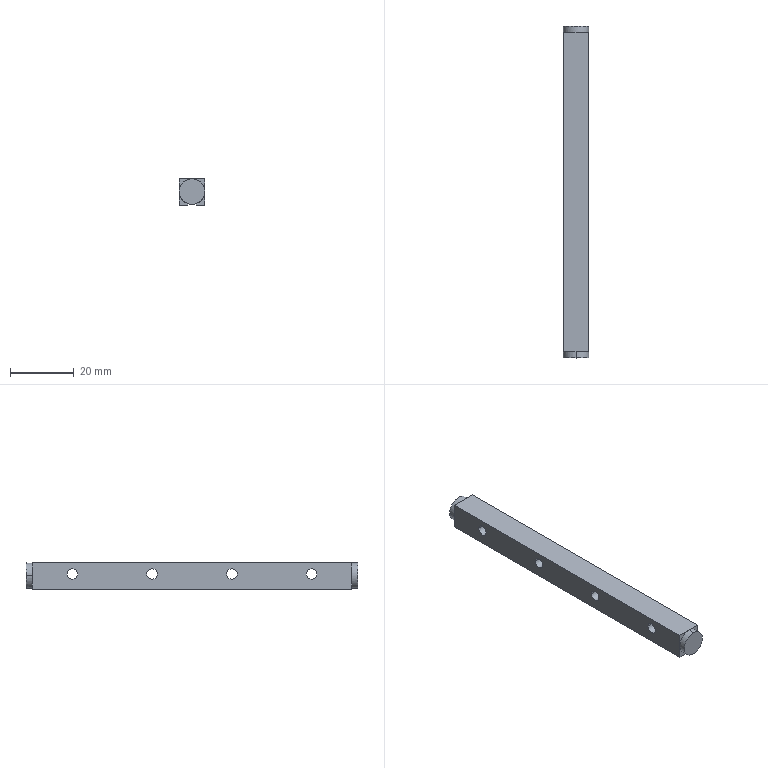Part | NX | 1 solid | 43 faces | box 8 x 104 x 8.3 mm | volume 6121 mm3 | plane 23 | cylinder 20 | commonest cylinder face diameters 3.3 x8 6 x8 8 x4
STEP:
#1=CARTESIAN_POINT('',(4.995,0.,-7.874));
#2=VERTEX_POINT('',#1);
#3=CARTESIAN_POINT('',(8.,0.,-4.));
#4=VERTEX_POINT('',#3);
#5=CARTESIAN_POINT('',(4.,0.,-4.));
#6=DIRECTION('',(0.,-1.,0.));
#7=DIRECTION('',(0.2489,0.,-0.9685));
#8=AXIS2_PLACEMENT_3D('',#5,#6,#7);
#9=CIRCLE('',#8,4.);
#10=EDGE_CURVE('',#2,#4,#9,.T.);
#11=ORIENTED_EDGE('',*,*,#10,.F.);
#12=CARTESIAN_POINT('',(5.421,0.,-8.3));
#13=VERTEX_POINT('',#12);
#14=CARTESIAN_POINT('',(5.421,0.,-8.3));
#15=DIRECTION('',(-0.7071,0.,0.7071));
#16=VECTOR('',#15,1000.);
#17=LINE('',#14,#16);
#18=EDGE_CURVE('',#13,#2,#17,.T.);
#19=ORIENTED_EDGE('',*,*,#18,.F.);
#20=CARTESIAN_POINT('',(8.,0.,-8.3));
#21=VERTEX_POINT('',#20);
#22=CARTESIAN_POINT('',(5.421,0.,-8.3));
#23=DIRECTION('',(1.,0.,0.));
#24=VECTOR('',#23,1000.);
#25=LINE('',#22,#24);
#26=EDGE_CURVE('',#13,#21,#25,.T.);
#27=ORIENTED_EDGE('',*,*,#26,.T.);
#28=CARTESIAN_POINT('',(8.,0.,-8.3));
#29=DIRECTION('',(0.,0.,1.));
#30=VECTOR('',#29,1000.);
#31=LINE('',#28,#30);
#32=EDGE_CURVE('',#21,#4,#31,.T.);
#33=ORIENTED_EDGE('',*,*,#32,.T.);
#34=EDGE_LOOP('',(#11,#19,#27,#33));
#35=FACE_BOUND('',#34,.T.);
#36=CARTESIAN_POINT('',(0.,0.,0.));
#37=DIRECTION('',(0.,1.,0.));
#38=DIRECTION('',(1.,0.,0.));
#39=AXIS2_PLACEMENT_3D('',#36,#37,#38);
#40=PLANE('',#39);
#41=ADVANCED_FACE('',(#35),#40,.F.);
#42=CARTESIAN_POINT('',(4.,-2.,0.));
#43=VERTEX_POINT('',#42);
#44=CARTESIAN_POINT('',(4.,-2.,-8.));
#45=VERTEX_POINT('',#44);
#46=CARTESIAN_POINT('',(4.,-2.,-4.));
#47=DIRECTION('',(0.,1.,0.));
#48=DIRECTION('',(0.,0.,1.));
#49=AXIS2_PLACEMENT_3D('',#46,#47,#48);
#50=CIRCLE('',#49,4.);
#51=EDGE_CURVE('',#43,#45,#50,.T.);
#52=ORIENTED_EDGE('',*,*,#51,.T.);
#53=CARTESIAN_POINT('',(4.,0.,-8.));
#54=VERTEX_POINT('',#53);
#55=CARTESIAN_POINT('',(4.,0.,-8.));
#56=DIRECTION('',(0.,-1.,0.));
#57=VECTOR('',#56,1000.);
#58=LINE('',#55,#57);
#59=EDGE_CURVE('',#45,#54,#58,.F.);
#60=ORIENTED_EDGE('',*,*,#59,.T.);
#61=CARTESIAN_POINT('',(4.,0.,-4.));
#62=DIRECTION('',(0.,-1.,0.));
#63=DIRECTION('',(-0.2489,0.,-0.9685));
#64=AXIS2_PLACEMENT_3D('',#61,#62,#63);
#65=CIRCLE('',#64,4.);
#66=EDGE_CURVE('',#54,#2,#65,.T.);
#67=ORIENTED_EDGE('',*,*,#66,.T.);
#68=ORIENTED_EDGE('',*,*,#10,.T.);
#69=CARTESIAN_POINT('',(4.,0.,0.));
#70=VERTEX_POINT('',#69);
#71=CARTESIAN_POINT('',(4.,0.,-4.));
#72=DIRECTION('',(0.,-1.,0.));
#73=DIRECTION('',(1.,0.,0.));
#74=AXIS2_PLACEMENT_3D('',#71,#72,#73);
#75=CIRCLE('',#74,4.);
#76=EDGE_CURVE('',#4,#70,#75,.T.);
#77=ORIENTED_EDGE('',*,*,#76,.T.);
#78=CARTESIAN_POINT('',(4.,0.,0.));
#79=DIRECTION('',(0.,-1.,0.));
#80=VECTOR('',#79,1000.);
#81=LINE('',#78,#80);
#82=EDGE_CURVE('',#43,#70,#81,.F.);
#83=ORIENTED_EDGE('',*,*,#82,.F.);
#84=EDGE_LOOP('',(#52,#60,#67,#68,#77,#83));
#85=FACE_BOUND('',#84,.T.);
#86=CARTESIAN_POINT('',(4.,0.,-4.));
#87=DIRECTION('',(0.,-1.,0.));
#88=DIRECTION('',(0.,0.,-1.));
#89=AXIS2_PLACEMENT_3D('',#86,#87,#88);
#90=CYLINDRICAL_SURFACE('',#89,4.);
#91=ADVANCED_FACE('',(#85),#90,.T.);
#92=CARTESIAN_POINT('',(4.,0.,-6.879));
#93=VERTEX_POINT('',#92);
#94=CARTESIAN_POINT('',(3.005,0.,-7.874));
#95=VERTEX_POINT('',#94);
#96=CARTESIAN_POINT('',(4.,0.,-6.879));
#97=DIRECTION('',(-0.7071,0.,-0.7071));
#98=VECTOR('',#97,1000.);
#99=LINE('',#96,#98);
#100=EDGE_CURVE('',#93,#95,#99,.T.);
#101=ORIENTED_EDGE('',*,*,#100,.F.);
#102=CARTESIAN_POINT('',(4.995,0.,-7.874));
#103=DIRECTION('',(-0.7071,0.,0.7071));
#104=VECTOR('',#103,1000.);
#105=LINE('',#102,#104);
#106=EDGE_CURVE('',#2,#93,#105,.T.);
#107=ORIENTED_EDGE('',*,*,#106,.F.);
#108=ORIENTED_EDGE('',*,*,#66,.F.);
#109=CARTESIAN_POINT('',(4.,0.,-4.));
#110=DIRECTION('',(0.,-1.,0.));
#111=DIRECTION('',(-0.2489,0.,-0.9685));
#112=AXIS2_PLACEMENT_3D('',#109,#110,#111);
#113=CIRCLE('',#112,4.);
#114=EDGE_CURVE('',#95,#54,#113,.T.);
#115=ORIENTED_EDGE('',*,*,#114,.F.);
#116=EDGE_LOOP('',(#101,#107,#108,#115));
#117=FACE_BOUND('',#116,.T.);
#118=CARTESIAN_POINT('',(0.,0.,0.));
#119=DIRECTION('',(0.,-1.,0.));
#120=DIRECTION('',(0.,0.,-1.));
#121=AXIS2_PLACEMENT_3D('',#118,#119,#120);
#122=PLANE('',#121);
#123=ADVANCED_FACE('',(#117),#122,.F.);
#124=ORIENTED_EDGE('',*,*,#100,.T.);
#125=CARTESIAN_POINT('',(2.579,0.,-8.3));
#126=VERTEX_POINT('',#125);
#127=CARTESIAN_POINT('',(3.005,0.,-7.874));
#128=DIRECTION('',(-0.7071,0.,-0.7071));
#129=VECTOR('',#128,1000.);
#130=LINE('',#127,#129);
#131=EDGE_CURVE('',#95,#126,#130,.T.);
#132=ORIENTED_EDGE('',*,*,#131,.T.);
#133=CARTESIAN_POINT('',(2.579,100.,-8.3));
#134=VERTEX_POINT('',#133);
#135=CARTESIAN_POINT('',(2.579,100.,-8.3));
#136=DIRECTION('',(0.,-1.,0.));
#137=VECTOR('',#136,1000.);
#138=LINE('',#135,#137);
#139=EDGE_CURVE('',#134,#126,#138,.T.);
#140=ORIENTED_EDGE('',*,*,#139,.F.);
#141=CARTESIAN_POINT('',(3.005,100.,-7.874));
#142=VERTEX_POINT('',#141);
#143=CARTESIAN_POINT('',(2.579,100.,-8.3));
#144=DIRECTION('',(0.7071,0.,0.7071));
#145=VECTOR('',#144,1000.);
#146=LINE('',#143,#145);
#147=EDGE_CURVE('',#134,#142,#146,.T.);
#148=ORIENTED_EDGE('',*,*,#147,.T.);
#149=CARTESIAN_POINT('',(4.,100.,-6.879));
#150=VERTEX_POINT('',#149);
#151=CARTESIAN_POINT('',(3.005,100.,-7.874));
#152=DIRECTION('',(0.7071,0.,0.7071));
#153=VECTOR('',#152,1000.);
#154=LINE('',#151,#153);
#155=EDGE_CURVE('',#142,#150,#154,.T.);
#156=ORIENTED_EDGE('',*,*,#155,.T.);
#157=CARTESIAN_POINT('',(4.,0.,-6.879));
#158=DIRECTION('',(0.,1.,0.));
#159=VECTOR('',#158,1000.);
#160=LINE('',#157,#159);
#161=EDGE_CURVE('',#93,#150,#160,.T.);
#162=ORIENTED_EDGE('',*,*,#161,.F.);
#163=EDGE_LOOP('',(#124,#132,#140,#148,#156,#162));
#164=FACE_BOUND('',#163,.T.);
#165=CARTESIAN_POINT('',(1.879,100.,-9.));
#166=DIRECTION('',(-0.7071,0.,0.7071));
#167=DIRECTION('',(0.,1.,0.));
#168=AXIS2_PLACEMENT_3D('',#165,#166,#167);
#169=PLANE('',#168);
#170=ADVANCED_FACE('',(#164),#169,.F.);
#171=ORIENTED_EDGE('',*,*,#106,.T.);
#172=ORIENTED_EDGE('',*,*,#161,.T.);
#173=CARTESIAN_POINT('',(4.995,100.,-7.874));
#174=VERTEX_POINT('',#173);
#175=CARTESIAN_POINT('',(4.,100.,-6.879));
#176=DIRECTION('',(0.7071,0.,-0.7071));
#177=VECTOR('',#176,1000.);
#178=LINE('',#175,#177);
#179=EDGE_CURVE('',#150,#174,#178,.T.);
#180=ORIENTED_EDGE('',*,*,#179,.T.);
#181=CARTESIAN_POINT('',(5.421,100.,-8.3));
#182=VERTEX_POINT('',#181);
#183=CARTESIAN_POINT('',(4.995,100.,-7.874));
#184=DIRECTION('',(0.7071,0.,-0.7071));
#185=VECTOR('',#184,1000.);
#186=LINE('',#183,#185);
#187=EDGE_CURVE('',#174,#182,#186,.T.);
#188=ORIENTED_EDGE('',*,*,#187,.T.);
#189=CARTESIAN_POINT('',(5.421,100.,-8.3));
#190=DIRECTION('',(0.,-1.,0.));
#191=VECTOR('',#190,1000.);
#192=LINE('',#189,#191);
#193=EDGE_CURVE('',#182,#13,#192,.T.);
#194=ORIENTED_EDGE('',*,*,#193,.T.);
#195=ORIENTED_EDGE('',*,*,#18,.T.);
#196=EDGE_LOOP('',(#171,#172,#180,#188,#194,#195));
#197=FACE_BOUND('',#196,.T.);
#198=CARTESIAN_POINT('',(4.,100.,-6.879));
#199=DIRECTION('',(0.7071,0.,0.7071));
#200=DIRECTION('',(0.,-1.,0.));
#201=AXIS2_PLACEMENT_3D('',#198,#199,#200);
#202=PLANE('',#201);
#203=ADVANCED_FACE('',(#197),#202,.F.);
#204=ORIENTED_EDGE('',*,*,#193,.F.);
#205=CARTESIAN_POINT('',(8.,100.,-8.3));
#206=VERTEX_POINT('',#205);
#207=CARTESIAN_POINT('',(5.421,100.,-8.3));
#208=DIRECTION('',(1.,0.,0.));
#209=VECTOR('',#208,1000.);
#210=LINE('',#207,#209);
#211=EDGE_CURVE('',#182,#206,#210,.T.);
#212=ORIENTED_EDGE('',*,*,#211,.T.);
#213=CARTESIAN_POINT('',(8.,100.,-8.3));
#214=DIRECTION('',(0.,-1.,0.));
#215=VECTOR('',#214,1000.);
#216=LINE('',#213,#215);
#217=EDGE_CURVE('',#206,#21,#216,.T.);
#218=ORIENTED_EDGE('',*,*,#217,.T.);
#219=ORIENTED_EDGE('',*,*,#26,.F.);
#220=EDGE_LOOP('',(#204,#212,#218,#219));
#221=FACE_BOUND('',#220,.T.);
#222=CARTESIAN_POINT('',(8.,0.,-8.3));
#223=DIRECTION('',(0.,0.,-1.));
#224=DIRECTION('',(0.,-1.,0.));
#225=AXIS2_PLACEMENT_3D('',#222,#223,#224);
#226=PLANE('',#225);
#227=ADVANCED_FACE('',(#221),#226,.T.);
#228=CARTESIAN_POINT('',(8.,0.,0.));
#229=VERTEX_POINT('',#228);
#230=CARTESIAN_POINT('',(8.,0.,-4.));
#231=DIRECTION('',(0.,0.,1.));
#232=VECTOR('',#231,1000.);
#233=LINE('',#230,#232);
#234=EDGE_CURVE('',#4,#229,#233,.T.);
#235=ORIENTED_EDGE('',*,*,#234,.F.);
#236=ORIENTED_EDGE('',*,*,#32,.F.);
#237=ORIENTED_EDGE('',*,*,#217,.F.);
#238=CARTESIAN_POINT('',(8.,100.,-4.));
#239=VERTEX_POINT('',#238);
#240=CARTESIAN_POINT('',(8.,100.,-8.3));
#241=DIRECTION('',(0.,0.,1.));
#242=VECTOR('',#241,1000.);
#243=LINE('',#240,#242);
#244=EDGE_CURVE('',#206,#239,#243,.T.);
#245=ORIENTED_EDGE('',*,*,#244,.T.);
#246=CARTESIAN_POINT('',(8.,100.,0.));
#247=VERTEX_POINT('',#246);
#248=CARTESIAN_POINT('',(8.,100.,-4.));
#249=DIRECTION('',(0.,0.,1.));
#250=VECTOR('',#249,1000.);
#251=LINE('',#248,#250);
#252=EDGE_CURVE('',#239,#247,#251,.T.);
#253=ORIENTED_EDGE('',*,*,#252,.T.);
#254=CARTESIAN_POINT('',(8.,100.,0.));
#255=DIRECTION('',(0.,-1.,0.));
#256=VECTOR('',#255,1000.);
#257=LINE('',#254,#256);
#258=EDGE_CURVE('',#247,#229,#257,.T.);
#259=ORIENTED_EDGE('',*,*,#258,.T.);
#260=EDGE_LOOP('',(#235,#236,#237,#245,#253,#259));
#261=FACE_BOUND('',#260,.T.);
#262=CARTESIAN_POINT('',(8.,84.5,-3.5));
#263=VERTEX_POINT('',#262);
#264=CARTESIAN_POINT('',(8.,90.5,-3.5));
#265=VERTEX_POINT('',#264);
#266=CARTESIAN_POINT('',(8.,87.5,-3.5));
#267=DIRECTION('',(1.,0.,0.));
#268=DIRECTION('',(0.,1.,0.));
#269=AXIS2_PLACEMENT_3D('',#266,#267,#268);
#270=CIRCLE('',#269,3.);
#271=EDGE_CURVE('',#263,#265,#270,.T.);
#272=ORIENTED_EDGE('',*,*,#271,.F.);
#273=CARTESIAN_POINT('',(8.,87.5,-3.5));
#274=DIRECTION('',(1.,0.,0.));
#275=DIRECTION('',(0.,1.,0.));
#276=AXIS2_PLACEMENT_3D('',#273,#274,#275);
#277=CIRCLE('',#276,3.);
#278=EDGE_CURVE('',#265,#263,#277,.T.);
#279=ORIENTED_EDGE('',*,*,#278,.F.);
#280=EDGE_LOOP('',(#272,#279));
#281=FACE_BOUND('',#280,.T.);
#282=CARTESIAN_POINT('',(8.,59.5,-3.5));
#283=VERTEX_POINT('',#282);
#284=CARTESIAN_POINT('',(8.,65.5,-3.5));
#285=VERTEX_POINT('',#284);
#286=CARTESIAN_POINT('',(8.,62.5,-3.5));
#287=DIRECTION('',(1.,0.,0.));
#288=DIRECTION('',(0.,1.,0.));
#289=AXIS2_PLACEMENT_3D('',#286,#287,#288);
#290=CIRCLE('',#289,3.);
#291=EDGE_CURVE('',#283,#285,#290,.T.);
#292=ORIENTED_EDGE('',*,*,#291,.F.);
#293=CARTESIAN_POINT('',(8.,62.5,-3.5));
#294=DIRECTION('',(1.,0.,0.));
#295=DIRECTION('',(0.,1.,0.));
#296=AXIS2_PLACEMENT_3D('',#293,#294,#295);
#297=CIRCLE('',#296,3.);
#298=EDGE_CURVE('',#285,#283,#297,.T.);
#299=ORIENTED_EDGE('',*,*,#298,.F.);
#300=EDGE_LOOP('',(#292,#299));
#301=FACE_BOUND('',#300,.T.);
#302=CARTESIAN_POINT('',(8.,40.5,-3.5));
#303=VERTEX_POINT('',#302);
#304=CARTESIAN_POINT('',(8.,34.5,-3.5));
#305=VERTEX_POINT('',#304);
#306=CARTESIAN_POINT('',(8.,37.5,-3.5));
#307=DIRECTION('',(1.,0.,0.));
#308=DIRECTION('',(0.,1.,0.));
#309=AXIS2_PLACEMENT_3D('',#306,#307,#308);
#310=CIRCLE('',#309,3.);
#311=EDGE_CURVE('',#303,#305,#310,.T.);
#312=ORIENTED_EDGE('',*,*,#311,.F.);
#313=CARTESIAN_POINT('',(8.,37.5,-3.5));
#314=DIRECTION('',(1.,0.,0.));
#315=DIRECTION('',(0.,1.,0.));
#316=AXIS2_PLACEMENT_3D('',#313,#314,#315);
#317=CIRCLE('',#316,3.);
#318=EDGE_CURVE('',#305,#303,#317,.T.);
#319=ORIENTED_EDGE('',*,*,#318,.F.);
#320=EDGE_LOOP('',(#312,#319));
#321=FACE_BOUND('',#320,.T.);
#322=CARTESIAN_POINT('',(8.,9.5,-3.5));
#323=VERTEX_POINT('',#322);
#324=CARTESIAN_POINT('',(8.,15.5,-3.5));
#325=VERTEX_POINT('',#324);
#326=CARTESIAN_POINT('',(8.,12.5,-3.5));
#327=DIRECTION('',(1.,0.,0.));
#328=DIRECTION('',(0.,1.,0.));
#329=AXIS2_PLACEMENT_3D('',#326,#327,#328);
#330=CIRCLE('',#329,3.);
#331=EDGE_CURVE('',#323,#325,#330,.T.);
#332=ORIENTED_EDGE('',*,*,#331,.F.);
#333=CARTESIAN_POINT('',(8.,12.5,-3.5));
#334=DIRECTION('',(1.,0.,0.));
#335=DIRECTION('',(0.,1.,0.));
#336=AXIS2_PLACEMENT_3D('',#333,#334,#335);
#337=CIRCLE('',#336,3.);
#338=EDGE_CURVE('',#325,#323,#337,.T.);
#339=ORIENTED_EDGE('',*,*,#338,.F.);
#340=EDGE_LOOP('',(#332,#339));
#341=FACE_BOUND('',#340,.T.);
#342=CARTESIAN_POINT('',(8.,0.,0.));
#343=DIRECTION('',(1.,0.,0.));
#344=DIRECTION('',(0.,1.,0.));
#345=AXIS2_PLACEMENT_3D('',#342,#343,#344);
#346=PLANE('',#345);
#347=ADVANCED_FACE('',(#261,#281,#301,#321,#341),#346,.T.);
#348=ORIENTED_EDGE('',*,*,#76,.F.);
#349=ORIENTED_EDGE('',*,*,#234,.T.);
#350=CARTESIAN_POINT('',(8.,0.,0.));
#351=DIRECTION('',(-1.,0.,0.));
#352=VECTOR('',#351,1000.);
#353=LINE('',#350,#352);
#354=EDGE_CURVE('',#229,#70,#353,.T.);
#355=ORIENTED_EDGE('',*,*,#354,.T.);
#356=EDGE_LOOP('',(#348,#349,#355));
#357=FACE_BOUND('',#356,.T.);
#358=CARTESIAN_POINT('',(0.,0.,0.));
#359=DIRECTION('',(0.,1.,0.));
#360=DIRECTION('',(1.,0.,0.));
#361=AXIS2_PLACEMENT_3D('',#358,#359,#360);
#362=PLANE('',#361);
#363=ADVANCED_FACE('',(#357),#362,.F.);
#364=CARTESIAN_POINT('',(0.,0.,0.));
#365=VERTEX_POINT('',#364);
#366=CARTESIAN_POINT('',(4.,0.,0.));
#367=DIRECTION('',(-1.,0.,0.));
#368=VECTOR('',#367,1000.);
#369=LINE('',#366,#368);
#370=EDGE_CURVE('',#70,#365,#369,.T.);
#371=ORIENTED_EDGE('',*,*,#370,.F.);
#372=ORIENTED_EDGE('',*,*,#354,.F.);
#373=ORIENTED_EDGE('',*,*,#258,.F.);
#374=CARTESIAN_POINT('',(4.,100.,0.));
#375=VERTEX_POINT('',#374);
#376=CARTESIAN_POINT('',(8.,100.,0.));
#377=DIRECTION('',(-1.,0.,0.));
#378=VECTOR('',#377,1000.);
#379=LINE('',#376,#378);
#380=EDGE_CURVE('',#247,#375,#379,.T.);
#381=ORIENTED_EDGE('',*,*,#380,.T.);
#382=CARTESIAN_POINT('',(0.,100.,0.));
#383=VERTEX_POINT('',#382);
#384=CARTESIAN_POINT('',(4.,100.,0.));
#385=DIRECTION('',(-1.,0.,0.));
#386=VECTOR('',#385,1000.);
#387=LINE('',#384,#386);
#388=EDGE_CURVE('',#375,#383,#387,.T.);
#389=ORIENTED_EDGE('',*,*,#388,.T.);
#390=CARTESIAN_POINT('',(0.,100.,0.));
#391=DIRECTION('',(0.,-1.,0.));
#392=VECTOR('',#391,1000.);
#393=LINE('',#390,#392);
#394=EDGE_CURVE('',#383,#365,#393,.T.);
#395=ORIENTED_EDGE('',*,*,#394,.T.);
#396=EDGE_LOOP('',(#371,#372,#373,#381,#389,#395));
#397=FACE_BOUND('',#396,.T.);
#398=CARTESIAN_POINT('',(0.,0.,0.));
#399=DIRECTION('',(0.,0.,1.));
#400=DIRECTION('',(1.,0.,0.));
#401=AXIS2_PLACEMENT_3D('',#398,#399,#400);
#402=PLANE('',#401);
#403=ADVANCED_FACE('',(#397),#402,.T.);
#404=CARTESIAN_POINT('',(0.,0.,-4.));
#405=VERTEX_POINT('',#404);
#406=CARTESIAN_POINT('',(4.,0.,-4.));
#407=DIRECTION('',(0.,-1.,0.));
#408=DIRECTION('',(0.,0.,1.));
#409=AXIS2_PLACEMENT_3D('',#406,#407,#408);
#410=CIRCLE('',#409,4.);
#411=EDGE_CURVE('',#70,#405,#410,.T.);
#412=ORIENTED_EDGE('',*,*,#411,.F.);
#413=ORIENTED_EDGE('',*,*,#370,.T.);
#414=CARTESIAN_POINT('',(0.,0.,0.));
#415=DIRECTION('',(0.,0.,-1.));
#416=VECTOR('',#415,1000.);
#417=LINE('',#414,#416);
#418=EDGE_CURVE('',#365,#405,#417,.T.);
#419=ORIENTED_EDGE('',*,*,#418,.T.);
#420=EDGE_LOOP('',(#412,#413,#419));
#421=FACE_BOUND('',#420,.T.);
#422=CARTESIAN_POINT('',(0.,0.,0.));
#423=DIRECTION('',(0.,1.,0.));
#424=DIRECTION('',(1.,0.,0.));
#425=AXIS2_PLACEMENT_3D('',#422,#423,#424);
#426=PLANE('',#425);
#427=ADVANCED_FACE('',(#421),#426,.F.);
#428=CARTESIAN_POINT('',(4.9,9.5,-3.5));
#429=VERTEX_POINT('',#428);
#430=CARTESIAN_POINT('',(4.9,15.5,-3.5));
#431=VERTEX_POINT('',#430);
#432=CARTESIAN_POINT('',(4.9,12.5,-3.5));
#433=DIRECTION('',(-1.,0.,0.));
#434=DIRECTION('',(0.,-1.,0.));
#435=AXIS2_PLACEMENT_3D('',#432,#433,#434);
#436=CIRCLE('',#435,3.);
#437=EDGE_CURVE('',#429,#431,#436,.T.);
#438=ORIENTED_EDGE('',*,*,#437,.F.);
#439=CARTESIAN_POINT('',(4.9,12.5,-3.5));
#440=DIRECTION('',(-1.,0.,0.));
#441=DIRECTION('',(0.,-1.,0.));
#442=AXIS2_PLACEMENT_3D('',#439,#440,#441);
#443=CIRCLE('',#442,3.);
#444=EDGE_CURVE('',#431,#429,#443,.T.);
#445=ORIENTED_EDGE('',*,*,#444,.F.);
#446=EDGE_LOOP('',(#438,#445));
#447=FACE_BOUND('',#446,.T.);
#448=CARTESIAN_POINT('',(4.9,14.15,-3.5));
#449=VERTEX_POINT('',#448);
#450=CARTESIAN_POINT('',(4.9,10.85,-3.5));
#451=VERTEX_POINT('',#450);
#452=CARTESIAN_POINT('',(4.9,12.5,-3.5));
#453=DIRECTION('',(1.,0.,0.));
#454=DIRECTION('',(0.,1.,0.));
#455=AXIS2_PLACEMENT_3D('',#452,#453,#454);
#456=CIRCLE('',#455,1.65);
#457=EDGE_CURVE('',#449,#451,#456,.T.);
#458=ORIENTED_EDGE('',*,*,#457,.F.);
#459=CARTESIAN_POINT('',(4.9,12.5,-3.5));
#460=DIRECTION('',(1.,0.,0.));
#461=DIRECTION('',(0.,1.,0.));
#462=AXIS2_PLACEMENT_3D('',#459,#460,#461);
#463=CIRCLE('',#462,1.65);
#464=EDGE_CURVE('',#451,#449,#463,.T.);
#465=ORIENTED_EDGE('',*,*,#464,.F.);
#466=EDGE_LOOP('',(#458,#465));
#467=FACE_BOUND('',#466,.T.);
#468=CARTESIAN_POINT('',(4.9,12.5,-3.5));
#469=DIRECTION('',(1.,0.,0.));
#470=DIRECTION('',(0.,1.,0.));
#471=AXIS2_PLACEMENT_3D('',#468,#469,#470);
#472=PLANE('',#471);
#473=ADVANCED_FACE('',(#447,#467),#472,.T.);
#474=ORIENTED_EDGE('',*,*,#51,.F.);
#475=CARTESIAN_POINT('',(4.,-2.,-4.));
#476=DIRECTION('',(0.,1.,0.));
#477=DIRECTION('',(0.,0.,1.));
#478=AXIS2_PLACEMENT_3D('',#475,#476,#477);
#479=CIRCLE('',#478,4.);
#480=EDGE_CURVE('',#45,#43,#479,.T.);
#481=ORIENTED_EDGE('',*,*,#480,.F.);
#482=EDGE_LOOP('',(#474,#481));
#483=FACE_BOUND('',#482,.T.);
#484=CARTESIAN_POINT('',(0.,-2.,0.));
#485=DIRECTION('',(0.,-1.,0.));
#486=DIRECTION('',(0.,0.,-1.));
#487=AXIS2_PLACEMENT_3D('',#484,#485,#486);
#488=PLANE('',#487);
#489=ADVANCED_FACE('',(#483),#488,.T.);
#490=CARTESIAN_POINT('',(4.,0.,-4.));
#491=DIRECTION('',(0.,-1.,0.));
#492=DIRECTION('',(-1.,0.,0.));
#493=AXIS2_PLACEMENT_3D('',#490,#491,#492);
#494=CIRCLE('',#493,4.);
#495=EDGE_CURVE('',#405,#95,#494,.T.);
#496=ORIENTED_EDGE('',*,*,#495,.F.);
#497=CARTESIAN_POINT('',(0.,0.,-8.3));
#498=VERTEX_POINT('',#497);
#499=CARTESIAN_POINT('',(0.,0.,-4.));
#500=DIRECTION('',(0.,0.,-1.));
#501=VECTOR('',#500,1000.);
#502=LINE('',#499,#501);
#503=EDGE_CURVE('',#405,#498,#502,.T.);
#504=ORIENTED_EDGE('',*,*,#503,.T.);
#505=CARTESIAN_POINT('',(0.,0.,-8.3));
#506=DIRECTION('',(1.,0.,0.));
#507=VECTOR('',#506,1000.);
#508=LINE('',#505,#507);
#509=EDGE_CURVE('',#498,#126,#508,.T.);
#510=ORIENTED_EDGE('',*,*,#509,.T.);
#511=ORIENTED_EDGE('',*,*,#131,.F.);
#512=EDGE_LOOP('',(#496,#504,#510,#511));
#513=FACE_BOUND('',#512,.T.);
#514=CARTESIAN_POINT('',(0.,0.,0.));
#515=DIRECTION('',(0.,1.,0.));
#516=DIRECTION('',(1.,0.,0.));
#517=AXIS2_PLACEMENT_3D('',#514,#515,#516);
#518=PLANE('',#517);
#519=ADVANCED_FACE('',(#513),#518,.F.);
#520=ORIENTED_EDGE('',*,*,#139,.T.);
#521=ORIENTED_EDGE('',*,*,#509,.F.);
#522=CARTESIAN_POINT('',(0.,100.,-8.3));
#523=VERTEX_POINT('',#522);
#524=CARTESIAN_POINT('',(0.,100.,-8.3));
#525=DIRECTION('',(0.,-1.,0.));
#526=VECTOR('',#525,1000.);
#527=LINE('',#524,#526);
#528=EDGE_CURVE('',#523,#498,#527,.T.);
#529=ORIENTED_EDGE('',*,*,#528,.F.);
#530=CARTESIAN_POINT('',(0.,100.,-8.3));
#531=DIRECTION('',(1.,0.,0.));
#532=VECTOR('',#531,1000.);
#533=LINE('',#530,#532);
#534=EDGE_CURVE('',#523,#134,#533,.T.);
#535=ORIENTED_EDGE('',*,*,#534,.T.);
#536=EDGE_LOOP('',(#520,#521,#529,#535));
#537=FACE_BOUND('',#536,.T.);
#538=CARTESIAN_POINT('',(8.,0.,-8.3));
#539=DIRECTION('',(0.,0.,-1.));
#540=DIRECTION('',(0.,-1.,0.));
#541=AXIS2_PLACEMENT_3D('',#538,#539,#540);
#542=PLANE('',#541);
#543=ADVANCED_FACE('',(#537),#542,.T.);
#544=CARTESIAN_POINT('',(0.,100.,-4.));
#545=VERTEX_POINT('',#544);
#546=CARTESIAN_POINT('',(4.,100.,-4.));
#547=DIRECTION('',(0.,1.,0.));
#548=DIRECTION('',(-0.2489,0.,-0.9685));
#549=AXIS2_PLACEMENT_3D('',#546,#547,#548);
#550=CIRCLE('',#549,4.);
#551=EDGE_CURVE('',#142,#545,#550,.T.);
#552=ORIENTED_EDGE('',*,*,#551,.F.);
#553=ORIENTED_EDGE('',*,*,#147,.F.);
#554=ORIENTED_EDGE('',*,*,#534,.F.);
#555=CARTESIAN_POINT('',(0.,100.,-4.));
#556=DIRECTION('',(0.,0.,-1.));
#557=VECTOR('',#556,1000.);
#558=LINE('',#555,#557);
#559=EDGE_CURVE('',#545,#523,#558,.T.);
#560=ORIENTED_EDGE('',*,*,#559,.F.);
#561=EDGE_LOOP('',(#552,#553,#554,#560));
#562=FACE_BOUND('',#561,.T.);
#563=CARTESIAN_POINT('',(0.,100.,0.));
#564=DIRECTION('',(0.,1.,0.));
#565=DIRECTION('',(1.,0.,0.));
#566=AXIS2_PLACEMENT_3D('',#563,#564,#565);
#567=PLANE('',#566);
#568=ADVANCED_FACE('',(#562),#567,.T.);
#569=CARTESIAN_POINT('',(0.,102.,-4.));
#570=VERTEX_POINT('',#569);
#571=CARTESIAN_POINT('',(8.,102.,-4.));
#572=VERTEX_POINT('',#571);
#573=CARTESIAN_POINT('',(4.,102.,-4.));
#574=DIRECTION('',(0.,-1.,0.));
#575=DIRECTION('',(1.,0.,0.));
#576=AXIS2_PLACEMENT_3D('',#573,#574,#575);
#577=CIRCLE('',#576,4.);
#578=EDGE_CURVE('',#570,#572,#577,.T.);
#579=ORIENTED_EDGE('',*,*,#578,.T.);
#580=CARTESIAN_POINT('',(8.,100.,-4.));
#581=DIRECTION('',(0.,1.,0.));
#582=VECTOR('',#581,1000.);
#583=LINE('',#580,#582);
#584=EDGE_CURVE('',#572,#239,#583,.F.);
#585=ORIENTED_EDGE('',*,*,#584,.T.);
#586=CARTESIAN_POINT('',(4.,100.,-4.));
#587=DIRECTION('',(0.,1.,0.));
#588=DIRECTION('',(1.,0.,0.));
#589=AXIS2_PLACEMENT_3D('',#586,#587,#588);
#590=CIRCLE('',#589,4.);
#591=EDGE_CURVE('',#239,#174,#590,.T.);
#592=ORIENTED_EDGE('',*,*,#591,.T.);
#593=CARTESIAN_POINT('',(4.,100.,-4.));
#594=DIRECTION('',(0.,1.,0.));
#595=DIRECTION('',(0.2489,0.,-0.9685));
#596=AXIS2_PLACEMENT_3D('',#593,#594,#595);
#597=CIRCLE('',#596,4.);
#598=EDGE_CURVE('',#174,#142,#597,.T.);
#599=ORIENTED_EDGE('',*,*,#598,.T.);
#600=ORIENTED_EDGE('',*,*,#551,.T.);
#601=CARTESIAN_POINT('',(0.,100.,-4.));
#602=DIRECTION('',(0.,1.,0.));
#603=VECTOR('',#602,1000.);
#604=LINE('',#601,#603);
#605=EDGE_CURVE('',#570,#545,#604,.F.);
#606=ORIENTED_EDGE('',*,*,#605,.F.);
#607=EDGE_LOOP('',(#579,#585,#592,#599,#600,#606));
#608=FACE_BOUND('',#607,.T.);
#609=CARTESIAN_POINT('',(4.,100.,-4.));
#610=DIRECTION('',(0.,1.,0.));
#611=DIRECTION('',(-1.,0.,0.));
#612=AXIS2_PLACEMENT_3D('',#609,#610,#611);
#613=CYLINDRICAL_SURFACE('',#612,4.);
#614=ADVANCED_FACE('',(#608),#613,.T.);
#615=ORIENTED_EDGE('',*,*,#591,.F.);
#616=ORIENTED_EDGE('',*,*,#244,.F.);
#617=ORIENTED_EDGE('',*,*,#211,.F.);
#618=ORIENTED_EDGE('',*,*,#187,.F.);
#619=EDGE_LOOP('',(#615,#616,#617,#618));
#620=FACE_BOUND('',#619,.T.);
#621=CARTESIAN_POINT('',(0.,100.,0.));
#622=DIRECTION('',(0.,1.,0.));
#623=DIRECTION('',(1.,0.,0.));
#624=AXIS2_PLACEMENT_3D('',#621,#622,#623);
#625=PLANE('',#624);
#626=ADVANCED_FACE('',(#620),#625,.T.);
#627=CARTESIAN_POINT('',(4.9,34.5,-3.5));
#628=VERTEX_POINT('',#627);
#629=CARTESIAN_POINT('',(4.9,40.5,-3.5));
#630=VERTEX_POINT('',#629);
#631=CARTESIAN_POINT('',(4.9,37.5,-3.5));
#632=DIRECTION('',(-1.,0.,0.));
#633=DIRECTION('',(0.,-1.,0.));
#634=AXIS2_PLACEMENT_3D('',#631,#632,#633);
#635=CIRCLE('',#634,3.);
#636=EDGE_CURVE('',#628,#630,#635,.T.);
#637=ORIENTED_EDGE('',*,*,#636,.T.);
#638=CARTESIAN_POINT('',(-1.24,40.5,-3.5));
#639=DIRECTION('',(1.,0.,0.));
#640=VECTOR('',#639,1000.);
#641=LINE('',#638,#640);
#642=EDGE_CURVE('',#303,#630,#641,.F.);
#643=ORIENTED_EDGE('',*,*,#642,.F.);
#644=ORIENTED_EDGE('',*,*,#311,.T.);
#645=CARTESIAN_POINT('',(-1.24,34.5,-3.5));
#646=DIRECTION('',(1.,0.,0.));
#647=VECTOR('',#646,1000.);
#648=LINE('',#645,#647);
#649=EDGE_CURVE('',#305,#628,#648,.F.);
#650=ORIENTED_EDGE('',*,*,#649,.T.);
#651=EDGE_LOOP('',(#637,#643,#644,#650));
#652=FACE_BOUND('',#651,.T.);
#653=CARTESIAN_POINT('',(-1.24,37.5,-3.5));
#654=DIRECTION('',(1.,0.,0.));
#655=DIRECTION('',(0.,-1.,0.));
#656=AXIS2_PLACEMENT_3D('',#653,#654,#655);
#657=CYLINDRICAL_SURFACE('',#656,3.);
#658=ADVANCED_FACE('',(#652),#657,.F.);
#659=CARTESIAN_POINT('',(4.,100.,-4.));
#660=DIRECTION('',(0.,1.,0.));
#661=DIRECTION('',(-1.,0.,0.));
#662=AXIS2_PLACEMENT_3D('',#659,#660,#661);
#663=CIRCLE('',#662,4.);
#664=EDGE_CURVE('',#545,#375,#663,.T.);
#665=ORIENTED_EDGE('',*,*,#664,.F.);
#666=CARTESIAN_POINT('',(0.,100.,0.));
#667=DIRECTION('',(0.,0.,-1.));
#668=VECTOR('',#667,1000.);
#669=LINE('',#666,#668);
#670=EDGE_CURVE('',#383,#545,#669,.T.);
#671=ORIENTED_EDGE('',*,*,#670,.F.);
#672=ORIENTED_EDGE('',*,*,#388,.F.);
#673=EDGE_LOOP('',(#665,#671,#672));
#674=FACE_BOUND('',#673,.T.);
#675=CARTESIAN_POINT('',(0.,100.,0.));
#676=DIRECTION('',(0.,1.,0.));
#677=DIRECTION('',(1.,0.,0.));
#678=AXIS2_PLACEMENT_3D('',#675,#676,#677);
#679=PLANE('',#678);
#680=ADVANCED_FACE('',(#674),#679,.T.);
#681=ORIENTED_EDGE('',*,*,#503,.F.);
#682=ORIENTED_EDGE('',*,*,#418,.F.);
#683=ORIENTED_EDGE('',*,*,#394,.F.);
#684=ORIENTED_EDGE('',*,*,#670,.T.);
#685=ORIENTED_EDGE('',*,*,#559,.T.);
#686=ORIENTED_EDGE('',*,*,#528,.T.);
#687=EDGE_LOOP('',(#681,#682,#683,#684,#685,#686));
#688=FACE_BOUND('',#687,.T.);
#689=CARTESIAN_POINT('',(0.,89.15,-3.5));
#690=VERTEX_POINT('',#689);
#691=CARTESIAN_POINT('',(0.,85.85,-3.5));
#692=VERTEX_POINT('',#691);
#693=CARTESIAN_POINT('',(0.,87.5,-3.5));
#694=DIRECTION('',(-1.,0.,0.));
#695=DIRECTION('',(0.,-1.,0.));
#696=AXIS2_PLACEMENT_3D('',#693,#694,#695);
#697=CIRCLE('',#696,1.65);
#698=EDGE_CURVE('',#690,#692,#697,.T.);
#699=ORIENTED_EDGE('',*,*,#698,.F.);
#700=CARTESIAN_POINT('',(0.,87.5,-3.5));
#701=DIRECTION('',(-1.,0.,0.));
#702=DIRECTION('',(0.,-1.,0.));
#703=AXIS2_PLACEMENT_3D('',#700,#701,#702);
#704=CIRCLE('',#703,1.65);
#705=EDGE_CURVE('',#692,#690,#704,.T.);
#706=ORIENTED_EDGE('',*,*,#705,.F.);
#707=EDGE_LOOP('',(#699,#706));
#708=FACE_BOUND('',#707,.T.);
#709=CARTESIAN_POINT('',(0.,64.15,-3.5));
#710=VERTEX_POINT('',#709);
#711=CARTESIAN_POINT('',(0.,60.85,-3.5));
#712=VERTEX_POINT('',#711);
#713=CARTESIAN_POINT('',(0.,62.5,-3.5));
#714=DIRECTION('',(-1.,0.,0.));
#715=DIRECTION('',(0.,-1.,0.));
#716=AXIS2_PLACEMENT_3D('',#713,#714,#715);
#717=CIRCLE('',#716,1.65);
#718=EDGE_CURVE('',#710,#712,#717,.T.);
#719=ORIENTED_EDGE('',*,*,#718,.F.);
#720=CARTESIAN_POINT('',(0.,62.5,-3.5));
#721=DIRECTION('',(-1.,0.,0.));
#722=DIRECTION('',(0.,-1.,0.));
#723=AXIS2_PLACEMENT_3D('',#720,#721,#722);
#724=CIRCLE('',#723,1.65);
#725=EDGE_CURVE('',#712,#710,#724,.T.);
#726=ORIENTED_EDGE('',*,*,#725,.F.);
#727=EDGE_LOOP('',(#719,#726));
#728=FACE_BOUND('',#727,.T.);
#729=CARTESIAN_POINT('',(0.,35.85,-3.5));
#730=VERTEX_POINT('',#729);
#731=CARTESIAN_POINT('',(0.,39.15,-3.5));
#732=VERTEX_POINT('',#731);
#733=CARTESIAN_POINT('',(0.,37.5,-3.5));
#734=DIRECTION('',(-1.,0.,0.));
#735=DIRECTION('',(0.,-1.,0.));
#736=AXIS2_PLACEMENT_3D('',#733,#734,#735);
#737=CIRCLE('',#736,1.65);
#738=EDGE_CURVE('',#730,#732,#737,.T.);
#739=ORIENTED_EDGE('',*,*,#738,.F.);
#740=CARTESIAN_POINT('',(0.,37.5,-3.5));
#741=DIRECTION('',(-1.,0.,0.));
#742=DIRECTION('',(0.,-1.,0.));
#743=AXIS2_PLACEMENT_3D('',#740,#741,#742);
#744=CIRCLE('',#743,1.65);
#745=EDGE_CURVE('',#732,#730,#744,.T.);
#746=ORIENTED_EDGE('',*,*,#745,.F.);
#747=EDGE_LOOP('',(#739,#746));
#748=FACE_BOUND('',#747,.T.);
#749=CARTESIAN_POINT('',(0.,14.15,-3.5));
#750=VERTEX_POINT('',#749);
#751=CARTESIAN_POINT('',(0.,10.85,-3.5));
#752=VERTEX_POINT('',#751);
#753=CARTESIAN_POINT('',(0.,12.5,-3.5));
#754=DIRECTION('',(-1.,0.,0.));
#755=DIRECTION('',(0.,-1.,0.));
#756=AXIS2_PLACEMENT_3D('',#753,#754,#755);
#757=CIRCLE('',#756,1.65);
#758=EDGE_CURVE('',#750,#752,#757,.T.);
#759=ORIENTED_EDGE('',*,*,#758,.F.);
#760=CARTESIAN_POINT('',(0.,12.5,-3.5));
#761=DIRECTION('',(-1.,0.,0.));
#762=DIRECTION('',(0.,-1.,0.));
#763=AXIS2_PLACEMENT_3D('',#760,#761,#762);
#764=CIRCLE('',#763,1.65);
#765=EDGE_CURVE('',#752,#750,#764,.T.);
#766=ORIENTED_EDGE('',*,*,#765,.F.);
#767=EDGE_LOOP('',(#759,#766));
#768=FACE_BOUND('',#767,.T.);
#769=CARTESIAN_POINT('',(0.,0.,-8.3));
#770=DIRECTION('',(-1.,0.,0.));
#771=DIRECTION('',(0.,0.,1.));
#772=AXIS2_PLACEMENT_3D('',#769,#770,#771);
#773=PLANE('',#772);
#774=ADVANCED_FACE('',(#688,#708,#728,#748,#768),#773,.T.);
#775=ORIENTED_EDGE('',*,*,#698,.T.);
#776=CARTESIAN_POINT('',(4.9,85.85,-3.5));
#777=VERTEX_POINT('',#776);
#778=CARTESIAN_POINT('',(-1.24,85.85,-3.5));
#779=DIRECTION('',(1.,0.,0.));
#780=VECTOR('',#779,1000.);
#781=LINE('',#778,#780);
#782=EDGE_CURVE('',#777,#692,#781,.F.);
#783=ORIENTED_EDGE('',*,*,#782,.F.);
#784=CARTESIAN_POINT('',(4.9,89.15,-3.5));
#785=VERTEX_POINT('',#784);
#786=CARTESIAN_POINT('',(4.9,87.5,-3.5));
#787=DIRECTION('',(1.,0.,0.));
#788=DIRECTION('',(0.,1.,0.));
#789=AXIS2_PLACEMENT_3D('',#786,#787,#788);
#790=CIRCLE('',#789,1.65);
#791=EDGE_CURVE('',#777,#785,#790,.T.);
#792=ORIENTED_EDGE('',*,*,#791,.T.);
#793=CARTESIAN_POINT('',(-1.24,89.15,-3.5));
#794=DIRECTION('',(1.,0.,0.));
#795=VECTOR('',#794,1000.);
#796=LINE('',#793,#795);
#797=EDGE_CURVE('',#785,#690,#796,.F.);
#798=ORIENTED_EDGE('',*,*,#797,.T.);
#799=EDGE_LOOP('',(#775,#783,#792,#798));
#800=FACE_BOUND('',#799,.T.);
#801=CARTESIAN_POINT('',(-1.24,87.5,-3.5));
#802=DIRECTION('',(1.,0.,0.));
#803=DIRECTION('',(0.,-1.,0.));
#804=AXIS2_PLACEMENT_3D('',#801,#802,#803);
#805=CYLINDRICAL_SURFACE('',#804,1.65);
#806=ADVANCED_FACE('',(#800),#805,.F.);
#807=ORIENTED_EDGE('',*,*,#457,.T.);
#808=CARTESIAN_POINT('',(-1.24,10.85,-3.5));
#809=DIRECTION('',(1.,0.,0.));
#810=VECTOR('',#809,1000.);
#811=LINE('',#808,#810);
#812=EDGE_CURVE('',#451,#752,#811,.F.);
#813=ORIENTED_EDGE('',*,*,#812,.T.);
#814=ORIENTED_EDGE('',*,*,#765,.T.);
#815=CARTESIAN_POINT('',(-1.24,14.15,-3.5));
#816=DIRECTION('',(1.,0.,0.));
#817=VECTOR('',#816,1000.);
#818=LINE('',#815,#817);
#819=EDGE_CURVE('',#449,#750,#818,.F.);
#820=ORIENTED_EDGE('',*,*,#819,.F.);
#821=EDGE_LOOP('',(#807,#813,#814,#820));
#822=FACE_BOUND('',#821,.T.);
#823=CARTESIAN_POINT('',(-1.24,12.5,-3.5));
#824=DIRECTION('',(1.,0.,0.));
#825=DIRECTION('',(0.,-1.,0.));
#826=AXIS2_PLACEMENT_3D('',#823,#824,#825);
#827=CYLINDRICAL_SURFACE('',#826,1.65);
#828=ADVANCED_FACE('',(#822),#827,.F.);
#829=CARTESIAN_POINT('',(4.9,84.5,-3.5));
#830=VERTEX_POINT('',#829);
#831=CARTESIAN_POINT('',(4.9,90.5,-3.5));
#832=VERTEX_POINT('',#831);
#833=CARTESIAN_POINT('',(4.9,87.5,-3.5));
#834=DIRECTION('',(-1.,0.,0.));
#835=DIRECTION('',(0.,-1.,0.));
#836=AXIS2_PLACEMENT_3D('',#833,#834,#835);
#837=CIRCLE('',#836,3.);
#838=EDGE_CURVE('',#830,#832,#837,.T.);
#839=ORIENTED_EDGE('',*,*,#838,.F.);
#840=CARTESIAN_POINT('',(4.9,87.5,-3.5));
#841=DIRECTION('',(-1.,0.,0.));
#842=DIRECTION('',(0.,-1.,0.));
#843=AXIS2_PLACEMENT_3D('',#840,#841,#842);
#844=CIRCLE('',#843,3.);
#845=EDGE_CURVE('',#832,#830,#844,.T.);
#846=ORIENTED_EDGE('',*,*,#845,.F.);
#847=EDGE_LOOP('',(#839,#846));
#848=FACE_BOUND('',#847,.T.);
#849=CARTESIAN_POINT('',(4.9,87.5,-3.5));
#850=DIRECTION('',(1.,0.,0.));
#851=DIRECTION('',(0.,1.,0.));
#852=AXIS2_PLACEMENT_3D('',#849,#850,#851);
#853=CIRCLE('',#852,1.65);
#854=EDGE_CURVE('',#785,#777,#853,.T.);
#855=ORIENTED_EDGE('',*,*,#854,.F.);
#856=ORIENTED_EDGE('',*,*,#791,.F.);
#857=EDGE_LOOP('',(#855,#856));
#858=FACE_BOUND('',#857,.T.);
#859=CARTESIAN_POINT('',(4.9,87.5,-3.5));
#860=DIRECTION('',(1.,0.,0.));
#861=DIRECTION('',(0.,1.,0.));
#862=AXIS2_PLACEMENT_3D('',#859,#860,#861);
#863=PLANE('',#862);
#864=ADVANCED_FACE('',(#848,#858),#863,.T.);
#865=ORIENTED_EDGE('',*,*,#271,.T.);
#866=CARTESIAN_POINT('',(-1.24,90.5,-3.5));
#867=DIRECTION('',(1.,0.,0.));
#868=VECTOR('',#867,1000.);
#869=LINE('',#866,#868);
#870=EDGE_CURVE('',#832,#265,#869,.T.);
#871=ORIENTED_EDGE('',*,*,#870,.F.);
#872=ORIENTED_EDGE('',*,*,#845,.T.);
#873=CARTESIAN_POINT('',(-1.24,84.5,-3.5));
#874=DIRECTION('',(1.,0.,0.));
#875=VECTOR('',#874,1000.);
#876=LINE('',#873,#875);
#877=EDGE_CURVE('',#830,#263,#876,.T.);
#878=ORIENTED_EDGE('',*,*,#877,.T.);
#879=EDGE_LOOP('',(#865,#871,#872,#878));
#880=FACE_BOUND('',#879,.T.);
#881=CARTESIAN_POINT('',(-1.24,87.5,-3.5));
#882=DIRECTION('',(1.,0.,0.));
#883=DIRECTION('',(0.,-1.,0.));
#884=AXIS2_PLACEMENT_3D('',#881,#882,#883);
#885=CYLINDRICAL_SURFACE('',#884,3.);
#886=ADVANCED_FACE('',(#880),#885,.F.);
#887=ORIENTED_EDGE('',*,*,#331,.T.);
#888=CARTESIAN_POINT('',(-1.24,15.5,-3.5));
#889=DIRECTION('',(1.,0.,0.));
#890=VECTOR('',#889,1000.);
#891=LINE('',#888,#890);
#892=EDGE_CURVE('',#431,#325,#891,.T.);
#893=ORIENTED_EDGE('',*,*,#892,.F.);
#894=ORIENTED_EDGE('',*,*,#444,.T.);
#895=CARTESIAN_POINT('',(-1.24,9.5,-3.5));
#896=DIRECTION('',(1.,0.,0.));
#897=VECTOR('',#896,1000.);
#898=LINE('',#895,#897);
#899=EDGE_CURVE('',#429,#323,#898,.T.);
#900=ORIENTED_EDGE('',*,*,#899,.T.);
#901=EDGE_LOOP('',(#887,#893,#894,#900));
#902=FACE_BOUND('',#901,.T.);
#903=CARTESIAN_POINT('',(-1.24,12.5,-3.5));
#904=DIRECTION('',(1.,0.,0.));
#905=DIRECTION('',(0.,-1.,0.));
#906=AXIS2_PLACEMENT_3D('',#903,#904,#905);
#907=CYLINDRICAL_SURFACE('',#906,3.);
#908=ADVANCED_FACE('',(#902),#907,.F.);
#909=ORIENTED_EDGE('',*,*,#718,.T.);
#910=CARTESIAN_POINT('',(4.9,60.85,-3.5));
#911=VERTEX_POINT('',#910);
#912=CARTESIAN_POINT('',(-1.24,60.85,-3.5));
#913=DIRECTION('',(1.,0.,0.));
#914=VECTOR('',#913,1000.);
#915=LINE('',#912,#914);
#916=EDGE_CURVE('',#911,#712,#915,.F.);
#917=ORIENTED_EDGE('',*,*,#916,.F.);
#918=CARTESIAN_POINT('',(4.9,64.15,-3.5));
#919=VERTEX_POINT('',#918);
#920=CARTESIAN_POINT('',(4.9,62.5,-3.5));
#921=DIRECTION('',(1.,0.,0.));
#922=DIRECTION('',(0.,1.,0.));
#923=AXIS2_PLACEMENT_3D('',#920,#921,#922);
#924=CIRCLE('',#923,1.65);
#925=EDGE_CURVE('',#911,#919,#924,.T.);
#926=ORIENTED_EDGE('',*,*,#925,.T.);
#927=CARTESIAN_POINT('',(-1.24,64.15,-3.5));
#928=DIRECTION('',(1.,0.,0.));
#929=VECTOR('',#928,1000.);
#930=LINE('',#927,#929);
#931=EDGE_CURVE('',#919,#710,#930,.F.);
#932=ORIENTED_EDGE('',*,*,#931,.T.);
#933=EDGE_LOOP('',(#909,#917,#926,#932));
#934=FACE_BOUND('',#933,.T.);
#935=CARTESIAN_POINT('',(-1.24,62.5,-3.5));
#936=DIRECTION('',(1.,0.,0.));
#937=DIRECTION('',(0.,-1.,0.));
#938=AXIS2_PLACEMENT_3D('',#935,#936,#937);
#939=CYLINDRICAL_SURFACE('',#938,1.65);
#940=ADVANCED_FACE('',(#934),#939,.F.);
#941=CARTESIAN_POINT('',(4.,100.,-4.));
#942=DIRECTION('',(0.,1.,0.));
#943=DIRECTION('',(0.,0.,1.));
#944=AXIS2_PLACEMENT_3D('',#941,#942,#943);
#945=CIRCLE('',#944,4.);
#946=EDGE_CURVE('',#375,#239,#945,.T.);
#947=ORIENTED_EDGE('',*,*,#946,.F.);
#948=ORIENTED_EDGE('',*,*,#380,.F.);
#949=ORIENTED_EDGE('',*,*,#252,.F.);
#950=EDGE_LOOP('',(#947,#948,#949));
#951=FACE_BOUND('',#950,.T.);
#952=CARTESIAN_POINT('',(0.,100.,0.));
#953=DIRECTION('',(0.,1.,0.));
#954=DIRECTION('',(1.,0.,0.));
#955=AXIS2_PLACEMENT_3D('',#952,#953,#954);
#956=PLANE('',#955);
#957=ADVANCED_FACE('',(#951),#956,.T.);
#958=CARTESIAN_POINT('',(4.9,59.5,-3.5));
#959=VERTEX_POINT('',#958);
#960=CARTESIAN_POINT('',(4.9,65.5,-3.5));
#961=VERTEX_POINT('',#960);
#962=CARTESIAN_POINT('',(4.9,62.5,-3.5));
#963=DIRECTION('',(-1.,0.,0.));
#964=DIRECTION('',(0.,-1.,0.));
#965=AXIS2_PLACEMENT_3D('',#962,#963,#964);
#966=CIRCLE('',#965,3.);
#967=EDGE_CURVE('',#959,#961,#966,.T.);
#968=ORIENTED_EDGE('',*,*,#967,.F.);
#969=CARTESIAN_POINT('',(4.9,62.5,-3.5));
#970=DIRECTION('',(-1.,0.,0.));
#971=DIRECTION('',(0.,-1.,0.));
#972=AXIS2_PLACEMENT_3D('',#969,#970,#971);
#973=CIRCLE('',#972,3.);
#974=EDGE_CURVE('',#961,#959,#973,.T.);
#975=ORIENTED_EDGE('',*,*,#974,.F.);
#976=EDGE_LOOP('',(#968,#975));
#977=FACE_BOUND('',#976,.T.);
#978=CARTESIAN_POINT('',(4.9,62.5,-3.5));
#979=DIRECTION('',(1.,0.,0.));
#980=DIRECTION('',(0.,1.,0.));
#981=AXIS2_PLACEMENT_3D('',#978,#979,#980);
#982=CIRCLE('',#981,1.65);
#983=EDGE_CURVE('',#919,#911,#982,.T.);
#984=ORIENTED_EDGE('',*,*,#983,.F.);
#985=ORIENTED_EDGE('',*,*,#925,.F.);
#986=EDGE_LOOP('',(#984,#985));
#987=FACE_BOUND('',#986,.T.);
#988=CARTESIAN_POINT('',(4.9,62.5,-3.5));
#989=DIRECTION('',(1.,0.,0.));
#990=DIRECTION('',(0.,1.,0.));
#991=AXIS2_PLACEMENT_3D('',#988,#989,#990);
#992=PLANE('',#991);
#993=ADVANCED_FACE('',(#977,#987),#992,.T.);
#994=ORIENTED_EDGE('',*,*,#967,.T.);
#995=CARTESIAN_POINT('',(-1.24,65.5,-3.5));
#996=DIRECTION('',(1.,0.,0.));
#997=VECTOR('',#996,1000.);
#998=LINE('',#995,#997);
#999=EDGE_CURVE('',#961,#285,#998,.T.);
#1000=ORIENTED_EDGE('',*,*,#999,.T.);
#1001=ORIENTED_EDGE('',*,*,#298,.T.);
#1002=CARTESIAN_POINT('',(-1.24,59.5,-3.5));
#1003=DIRECTION('',(1.,0.,0.));
#1004=VECTOR('',#1003,1000.);
#1005=LINE('',#1002,#1004);
#1006=EDGE_CURVE('',#959,#283,#1005,.T.);
#1007=ORIENTED_EDGE('',*,*,#1006,.F.);
#1008=EDGE_LOOP('',(#994,#1000,#1001,#1007));
#1009=FACE_BOUND('',#1008,.T.);
#1010=CARTESIAN_POINT('',(-1.24,62.5,-3.5));
#1011=DIRECTION('',(1.,0.,0.));
#1012=DIRECTION('',(0.,-1.,0.));
#1013=AXIS2_PLACEMENT_3D('',#1010,#1011,#1012);
#1014=CYLINDRICAL_SURFACE('',#1013,3.);
#1015=ADVANCED_FACE('',(#1009),#1014,.F.);
#1016=ORIENTED_EDGE('',*,*,#155,.F.);
#1017=ORIENTED_EDGE('',*,*,#598,.F.);
#1018=ORIENTED_EDGE('',*,*,#179,.F.);
#1019=EDGE_LOOP('',(#1016,#1017,#1018));
#1020=FACE_BOUND('',#1019,.T.);
#1021=CARTESIAN_POINT('',(0.,100.,0.));
#1022=DIRECTION('',(0.,1.,0.));
#1023=DIRECTION('',(1.,0.,0.));
#1024=AXIS2_PLACEMENT_3D('',#1021,#1022,#1023);
#1025=PLANE('',#1024);
#1026=ADVANCED_FACE('',(#1020),#1025,.F.);
#1027=ORIENTED_EDGE('',*,*,#738,.T.);
#1028=CARTESIAN_POINT('',(4.9,39.15,-3.5));
#1029=VERTEX_POINT('',#1028);
#1030=CARTESIAN_POINT('',(-1.24,39.15,-3.5));
#1031=DIRECTION('',(1.,0.,0.));
#1032=VECTOR('',#1031,1000.);
#1033=LINE('',#1030,#1032);
#1034=EDGE_CURVE('',#1029,#732,#1033,.F.);
#1035=ORIENTED_EDGE('',*,*,#1034,.F.);
#1036=CARTESIAN_POINT('',(4.9,35.85,-3.5));
#1037=VERTEX_POINT('',#1036);
#1038=CARTESIAN_POINT('',(4.9,37.5,-3.5));
#1039=DIRECTION('',(1.,0.,0.));
#1040=DIRECTION('',(0.,1.,0.));
#1041=AXIS2_PLACEMENT_3D('',#1038,#1039,#1040);
#1042=CIRCLE('',#1041,1.65);
#1043=EDGE_CURVE('',#1029,#1037,#1042,.T.);
#1044=ORIENTED_EDGE('',*,*,#1043,.T.);
#1045=CARTESIAN_POINT('',(-1.24,35.85,-3.5));
#1046=DIRECTION('',(1.,0.,0.));
#1047=VECTOR('',#1046,1000.);
#1048=LINE('',#1045,#1047);
#1049=EDGE_CURVE('',#1037,#730,#1048,.F.);
#1050=ORIENTED_EDGE('',*,*,#1049,.T.);
#1051=EDGE_LOOP('',(#1027,#1035,#1044,#1050));
#1052=FACE_BOUND('',#1051,.T.);
#1053=CARTESIAN_POINT('',(-1.24,37.5,-3.5));
#1054=DIRECTION('',(1.,0.,0.));
#1055=DIRECTION('',(0.,-1.,0.));
#1056=AXIS2_PLACEMENT_3D('',#1053,#1054,#1055);
#1057=CYLINDRICAL_SURFACE('',#1056,1.65);
#1058=ADVANCED_FACE('',(#1052),#1057,.F.);
#1059=ORIENTED_EDGE('',*,*,#578,.F.);
#1060=CARTESIAN_POINT('',(4.,102.,-4.));
#1061=DIRECTION('',(0.,-1.,0.));
#1062=DIRECTION('',(1.,0.,0.));
#1063=AXIS2_PLACEMENT_3D('',#1060,#1061,#1062);
#1064=CIRCLE('',#1063,4.);
#1065=EDGE_CURVE('',#572,#570,#1064,.T.);
#1066=ORIENTED_EDGE('',*,*,#1065,.F.);
#1067=EDGE_LOOP('',(#1059,#1066));
#1068=FACE_BOUND('',#1067,.T.);
#1069=CARTESIAN_POINT('',(0.,102.,0.));
#1070=DIRECTION('',(0.,1.,0.));
#1071=DIRECTION('',(1.,0.,0.));
#1072=AXIS2_PLACEMENT_3D('',#1069,#1070,#1071);
#1073=PLANE('',#1072);
#1074=ADVANCED_FACE('',(#1068),#1073,.T.);
#1075=ORIENTED_EDGE('',*,*,#636,.F.);
#1076=CARTESIAN_POINT('',(4.9,37.5,-3.5));
#1077=DIRECTION('',(-1.,0.,0.));
#1078=DIRECTION('',(0.,-1.,0.));
#1079=AXIS2_PLACEMENT_3D('',#1076,#1077,#1078);
#1080=CIRCLE('',#1079,3.);
#1081=EDGE_CURVE('',#630,#628,#1080,.T.);
#1082=ORIENTED_EDGE('',*,*,#1081,.F.);
#1083=EDGE_LOOP('',(#1075,#1082));
#1084=FACE_BOUND('',#1083,.T.);
#1085=ORIENTED_EDGE('',*,*,#1043,.F.);
#1086=CARTESIAN_POINT('',(4.9,37.5,-3.5));
#1087=DIRECTION('',(1.,0.,0.));
#1088=DIRECTION('',(0.,1.,0.));
#1089=AXIS2_PLACEMENT_3D('',#1086,#1087,#1088);
#1090=CIRCLE('',#1089,1.65);
#1091=EDGE_CURVE('',#1037,#1029,#1090,.T.);
#1092=ORIENTED_EDGE('',*,*,#1091,.F.);
#1093=EDGE_LOOP('',(#1085,#1092));
#1094=FACE_BOUND('',#1093,.T.);
#1095=CARTESIAN_POINT('',(4.9,37.5,-3.5));
#1096=DIRECTION('',(1.,0.,0.));
#1097=DIRECTION('',(0.,1.,0.));
#1098=AXIS2_PLACEMENT_3D('',#1095,#1096,#1097);
#1099=PLANE('',#1098);
#1100=ADVANCED_FACE('',(#1084,#1094),#1099,.T.);
#1101=ORIENTED_EDGE('',*,*,#437,.T.);
#1102=ORIENTED_EDGE('',*,*,#892,.T.);
#1103=ORIENTED_EDGE('',*,*,#338,.T.);
#1104=ORIENTED_EDGE('',*,*,#899,.F.);
#1105=EDGE_LOOP('',(#1101,#1102,#1103,#1104));
#1106=FACE_BOUND('',#1105,.T.);
#1107=CARTESIAN_POINT('',(-1.24,12.5,-3.5));
#1108=DIRECTION('',(1.,0.,0.));
#1109=DIRECTION('',(0.,-1.,0.));
#1110=AXIS2_PLACEMENT_3D('',#1107,#1108,#1109);
#1111=CYLINDRICAL_SURFACE('',#1110,3.);
#1112=ADVANCED_FACE('',(#1106),#1111,.F.);
#1113=ORIENTED_EDGE('',*,*,#649,.F.);
#1114=ORIENTED_EDGE('',*,*,#318,.T.);
#1115=ORIENTED_EDGE('',*,*,#642,.T.);
#1116=ORIENTED_EDGE('',*,*,#1081,.T.);
#1117=EDGE_LOOP('',(#1113,#1114,#1115,#1116));
#1118=FACE_BOUND('',#1117,.T.);
#1119=CARTESIAN_POINT('',(-1.24,37.5,-3.5));
#1120=DIRECTION('',(1.,0.,0.));
#1121=DIRECTION('',(0.,-1.,0.));
#1122=AXIS2_PLACEMENT_3D('',#1119,#1120,#1121);
#1123=CYLINDRICAL_SURFACE('',#1122,3.);
#1124=ADVANCED_FACE('',(#1118),#1123,.F.);
#1125=ORIENTED_EDGE('',*,*,#291,.T.);
#1126=ORIENTED_EDGE('',*,*,#999,.F.);
#1127=ORIENTED_EDGE('',*,*,#974,.T.);
#1128=ORIENTED_EDGE('',*,*,#1006,.T.);
#1129=EDGE_LOOP('',(#1125,#1126,#1127,#1128));
#1130=FACE_BOUND('',#1129,.T.);
#1131=CARTESIAN_POINT('',(-1.24,62.5,-3.5));
#1132=DIRECTION('',(1.,0.,0.));
#1133=DIRECTION('',(0.,-1.,0.));
#1134=AXIS2_PLACEMENT_3D('',#1131,#1132,#1133);
#1135=CYLINDRICAL_SURFACE('',#1134,3.);
#1136=ADVANCED_FACE('',(#1130),#1135,.F.);
#1137=ORIENTED_EDGE('',*,*,#838,.T.);
#1138=ORIENTED_EDGE('',*,*,#870,.T.);
#1139=ORIENTED_EDGE('',*,*,#278,.T.);
#1140=ORIENTED_EDGE('',*,*,#877,.F.);
#1141=EDGE_LOOP('',(#1137,#1138,#1139,#1140));
#1142=FACE_BOUND('',#1141,.T.);
#1143=CARTESIAN_POINT('',(-1.24,87.5,-3.5));
#1144=DIRECTION('',(1.,0.,0.));
#1145=DIRECTION('',(0.,-1.,0.));
#1146=AXIS2_PLACEMENT_3D('',#1143,#1144,#1145);
#1147=CYLINDRICAL_SURFACE('',#1146,3.);
#1148=ADVANCED_FACE('',(#1142),#1147,.F.);
#1149=ORIENTED_EDGE('',*,*,#605,.T.);
#1150=ORIENTED_EDGE('',*,*,#664,.T.);
#1151=ORIENTED_EDGE('',*,*,#946,.T.);
#1152=ORIENTED_EDGE('',*,*,#584,.F.);
#1153=ORIENTED_EDGE('',*,*,#1065,.T.);
#1154=EDGE_LOOP('',(#1149,#1150,#1151,#1152,#1153));
#1155=FACE_BOUND('',#1154,.T.);
#1156=CARTESIAN_POINT('',(4.,100.,-4.));
#1157=DIRECTION('',(0.,1.,0.));
#1158=DIRECTION('',(-1.,0.,0.));
#1159=AXIS2_PLACEMENT_3D('',#1156,#1157,#1158);
#1160=CYLINDRICAL_SURFACE('',#1159,4.);
#1161=ADVANCED_FACE('',(#1155),#1160,.T.);
#1162=ORIENTED_EDGE('',*,*,#758,.T.);
#1163=ORIENTED_EDGE('',*,*,#812,.F.);
#1164=ORIENTED_EDGE('',*,*,#464,.T.);
#1165=ORIENTED_EDGE('',*,*,#819,.T.);
#1166=EDGE_LOOP('',(#1162,#1163,#1164,#1165));
#1167=FACE_BOUND('',#1166,.T.);
#1168=CARTESIAN_POINT('',(-1.24,12.5,-3.5));
#1169=DIRECTION('',(1.,0.,0.));
#1170=DIRECTION('',(0.,-1.,0.));
#1171=AXIS2_PLACEMENT_3D('',#1168,#1169,#1170);
#1172=CYLINDRICAL_SURFACE('',#1171,1.65);
#1173=ADVANCED_FACE('',(#1167),#1172,.F.);
#1174=ORIENTED_EDGE('',*,*,#1049,.F.);
#1175=ORIENTED_EDGE('',*,*,#1091,.T.);
#1176=ORIENTED_EDGE('',*,*,#1034,.T.);
#1177=ORIENTED_EDGE('',*,*,#745,.T.);
#1178=EDGE_LOOP('',(#1174,#1175,#1176,#1177));
#1179=FACE_BOUND('',#1178,.T.);
#1180=CARTESIAN_POINT('',(-1.24,37.5,-3.5));
#1181=DIRECTION('',(1.,0.,0.));
#1182=DIRECTION('',(0.,-1.,0.));
#1183=AXIS2_PLACEMENT_3D('',#1180,#1181,#1182);
#1184=CYLINDRICAL_SURFACE('',#1183,1.65);
#1185=ADVANCED_FACE('',(#1179),#1184,.F.);
#1186=ORIENTED_EDGE('',*,*,#983,.T.);
#1187=ORIENTED_EDGE('',*,*,#916,.T.);
#1188=ORIENTED_EDGE('',*,*,#725,.T.);
#1189=ORIENTED_EDGE('',*,*,#931,.F.);
#1190=EDGE_LOOP('',(#1186,#1187,#1188,#1189));
#1191=FACE_BOUND('',#1190,.T.);
#1192=CARTESIAN_POINT('',(-1.24,62.5,-3.5));
#1193=DIRECTION('',(1.,0.,0.));
#1194=DIRECTION('',(0.,-1.,0.));
#1195=AXIS2_PLACEMENT_3D('',#1192,#1193,#1194);
#1196=CYLINDRICAL_SURFACE('',#1195,1.65);
#1197=ADVANCED_FACE('',(#1191),#1196,.F.);
#1198=ORIENTED_EDGE('',*,*,#59,.F.);
#1199=ORIENTED_EDGE('',*,*,#480,.T.);
#1200=ORIENTED_EDGE('',*,*,#82,.T.);
#1201=ORIENTED_EDGE('',*,*,#411,.T.);
#1202=ORIENTED_EDGE('',*,*,#495,.T.);
#1203=ORIENTED_EDGE('',*,*,#114,.T.);
#1204=EDGE_LOOP('',(#1198,#1199,#1200,#1201,#1202,#1203));
#1205=FACE_BOUND('',#1204,.T.);
#1206=CARTESIAN_POINT('',(4.,0.,-4.));
#1207=DIRECTION('',(0.,-1.,0.));
#1208=DIRECTION('',(0.,0.,-1.));
#1209=AXIS2_PLACEMENT_3D('',#1206,#1207,#1208);
#1210=CYLINDRICAL_SURFACE('',#1209,4.);
#1211=ADVANCED_FACE('',(#1205),#1210,.T.);
#1212=ORIENTED_EDGE('',*,*,#854,.T.);
#1213=ORIENTED_EDGE('',*,*,#782,.T.);
#1214=ORIENTED_EDGE('',*,*,#705,.T.);
#1215=ORIENTED_EDGE('',*,*,#797,.F.);
#1216=EDGE_LOOP('',(#1212,#1213,#1214,#1215));
#1217=FACE_BOUND('',#1216,.T.);
#1218=CARTESIAN_POINT('',(-1.24,87.5,-3.5));
#1219=DIRECTION('',(1.,0.,0.));
#1220=DIRECTION('',(0.,-1.,0.));
#1221=AXIS2_PLACEMENT_3D('',#1218,#1219,#1220);
#1222=CYLINDRICAL_SURFACE('',#1221,1.65);
#1223=ADVANCED_FACE('',(#1217),#1222,.F.);
#1224=CLOSED_SHELL('',(#41,#91,#123,#170,#203,#227,#347,#363,#403,#427,#473,#489,#519,#543,#568,#614,#626,#658,#680,#774,#806,#828,#864,#886,#908,#940,#957,#993,#1015,#1026,#1058,#1074,#1100,#1112,#1124,#1136,#1148,#1161,#1173,#1185,#1197,#1211,#1223));
#1225=MANIFOLD_SOLID_BREP('',#1224);
#1226=(LENGTH_UNIT()NAMED_UNIT(*)SI_UNIT(.MILLI.,.METRE.));
#1227=UNCERTAINTY_MEASURE_WITH_UNIT(LENGTH_MEASURE(0.00001),#1226,'','');
#1228=(NAMED_UNIT(*)PLANE_ANGLE_UNIT()SI_UNIT($,.RADIAN.));
#1229=(NAMED_UNIT(*)SI_UNIT($,.STERADIAN.)SOLID_ANGLE_UNIT());
#1230=(GEOMETRIC_REPRESENTATION_CONTEXT(3)GLOBAL_UNCERTAINTY_ASSIGNED_CONTEXT((#1227))GLOBAL_UNIT_ASSIGNED_CONTEXT((#1226,#1228,#1229))REPRESENTATION_CONTEXT('',''));
#1231=ADVANCED_BREP_SHAPE_REPRESENTATION('',(#1225),#1230);